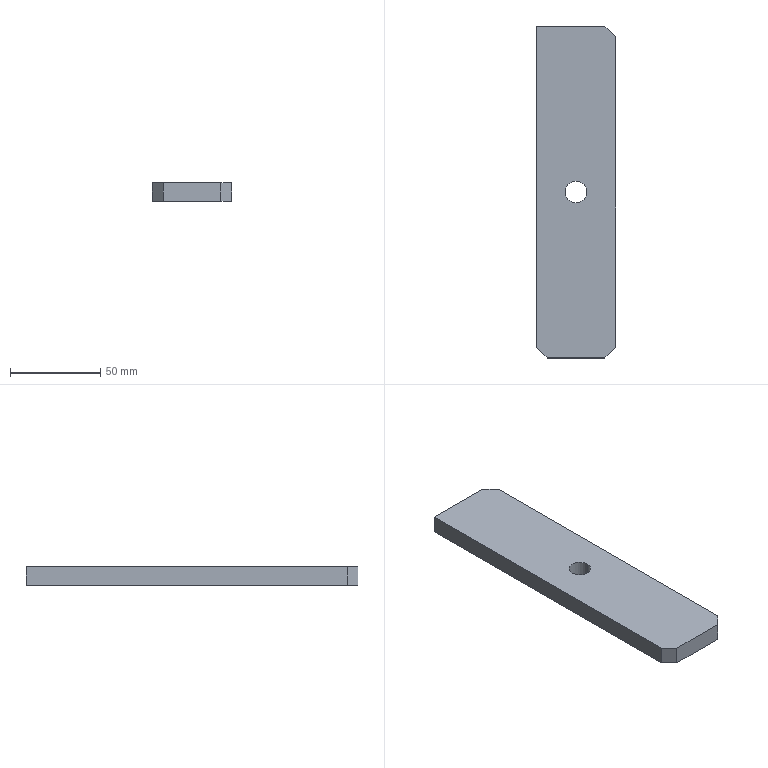Part | STEP file | PN_0011_plate_default_machined_ | 1 solid | 11 faces | box 44 x 184 x 10 mm | volume 79289 mm3 | plane 9 | cylinder 2 | commonest cylinder face diameters 12 x2
STEP:
#1=CARTESIAN_POINT('',(0.,0.,0.));
#2=DIRECTION('',(0.,0.,1.));
#3=DIRECTION('',(1.,0.,0.));
#4=AXIS2_PLACEMENT_3D('',#1,#2,#3);
#5=CARTESIAN_POINT('',(28.,92.,-10.));
#6=VERTEX_POINT('',#5);
#7=CARTESIAN_POINT('',(28.,92.,0.));
#8=VERTEX_POINT('',#7);
#9=CARTESIAN_POINT('',(28.,92.,0.));
#10=DIRECTION('',(0.,0.,1.));
#11=VECTOR('',#10,1.);
#12=LINE('',#9,#11);
#13=CARTESIAN_POINT('',(22.,92.,0.));
#14=DIRECTION('',(0.,0.,1.));
#15=DIRECTION('',(1.,0.,0.));
#16=AXIS2_PLACEMENT_3D('',#13,#14,#15);
#17=CYLINDRICAL_SURFACE('',#16,6.);
#18=CARTESIAN_POINT('',(6.283,0.));
#19=DIRECTION('',(0.,1.));
#20=VECTOR('',#19,1.);
#21=LINE('',#18,#20);
#22=(GEOMETRIC_REPRESENTATION_CONTEXT(2)PARAMETRIC_REPRESENTATION_CONTEXT()REPRESENTATION_CONTEXT('',''));
#23=DEFINITIONAL_REPRESENTATION('',(#21),#22);
#24=PCURVE('',#17,#23);
#25=CARTESIAN_POINT('',(22.,92.,0.));
#26=DIRECTION('',(0.,0.,1.));
#27=DIRECTION('',(1.,0.,0.));
#28=AXIS2_PLACEMENT_3D('',#25,#26,#27);
#29=CYLINDRICAL_SURFACE('',#28,6.);
#30=CARTESIAN_POINT('',(0.,0.));
#31=DIRECTION('',(0.,1.));
#32=VECTOR('',#31,1.);
#33=LINE('',#30,#32);
#34=(GEOMETRIC_REPRESENTATION_CONTEXT(2)PARAMETRIC_REPRESENTATION_CONTEXT()REPRESENTATION_CONTEXT('',''));
#35=DEFINITIONAL_REPRESENTATION('',(#33),#34);
#36=PCURVE('',#29,#35);
#37=SURFACE_CURVE('',#12,(#24,#36),.PCURVE_S1.);
#38=EDGE_CURVE('',#6,#8,#37,.T.);
#39=ORIENTED_EDGE('',*,*,#38,.T.);
#40=CARTESIAN_POINT('',(16.,92.,0.));
#41=VERTEX_POINT('',#40);
#42=CARTESIAN_POINT('',(22.,92.,0.));
#43=DIRECTION('',(0.,0.,1.));
#44=DIRECTION('',(1.,0.,0.));
#45=AXIS2_PLACEMENT_3D('',#42,#43,#44);
#46=CIRCLE('',#45,6.);
#47=CARTESIAN_POINT('',(0.,0.));
#48=DIRECTION('',(1.,0.));
#49=VECTOR('',#48,1.);
#50=LINE('',#47,#49);
#51=(GEOMETRIC_REPRESENTATION_CONTEXT(2)PARAMETRIC_REPRESENTATION_CONTEXT()REPRESENTATION_CONTEXT('',''));
#52=DEFINITIONAL_REPRESENTATION('',(#50),#51);
#53=PCURVE('',#17,#52);
#54=CARTESIAN_POINT('',(0.,0.,0.));
#55=DIRECTION('',(0.,0.,-1.));
#56=DIRECTION('',(-1.,0.,0.));
#57=AXIS2_PLACEMENT_3D('',#54,#55,#56);
#58=PLANE('',#57);
#59=CARTESIAN_POINT('',(-28.,92.));
#60=CARTESIAN_POINT('',(-28.,102.392));
#61=CARTESIAN_POINT('',(-19.,97.196));
#62=CARTESIAN_POINT('',(-10.,92.));
#63=CARTESIAN_POINT('',(-19.,86.804));
#64=CARTESIAN_POINT('',(-28.,81.608));
#65=CARTESIAN_POINT('',(-28.,92.));
#66=(BOUNDED_CURVE()B_SPLINE_CURVE(2,(#59,#60,#61,#62,#63,#64,#65),.UNSPECIFIED.,.T.,.F.)B_SPLINE_CURVE_WITH_KNOTS((1,2,2,2,2,1),(-2.094,0.,2.094,4.189,6.283,8.378),.UNSPECIFIED.)CURVE()GEOMETRIC_REPRESENTATION_ITEM()RATIONAL_B_SPLINE_CURVE((1.,0.5,1.,0.5,1.,0.5,1.))REPRESENTATION_ITEM(''));
#67=(GEOMETRIC_REPRESENTATION_CONTEXT(2)PARAMETRIC_REPRESENTATION_CONTEXT()REPRESENTATION_CONTEXT('',''));
#68=DEFINITIONAL_REPRESENTATION('',(#66),#67);
#69=PCURVE('',#58,#68);
#70=SURFACE_CURVE('',#46,(#53,#69),.PCURVE_S1.);
#71=EDGE_CURVE('',#41,#8,#70,.T.);
#72=ORIENTED_EDGE('',*,*,#71,.F.);
#73=CARTESIAN_POINT('',(16.,92.,-10.));
#74=VERTEX_POINT('',#73);
#75=CARTESIAN_POINT('',(16.,92.,0.));
#76=DIRECTION('',(0.,0.,1.));
#77=VECTOR('',#76,1.);
#78=LINE('',#75,#77);
#79=CARTESIAN_POINT('',(3.142,0.));
#80=DIRECTION('',(0.,1.));
#81=VECTOR('',#80,1.);
#82=LINE('',#79,#81);
#83=(GEOMETRIC_REPRESENTATION_CONTEXT(2)PARAMETRIC_REPRESENTATION_CONTEXT()REPRESENTATION_CONTEXT('',''));
#84=DEFINITIONAL_REPRESENTATION('',(#82),#83);
#85=PCURVE('',#17,#84);
#86=CARTESIAN_POINT('',(3.142,0.));
#87=DIRECTION('',(0.,1.));
#88=VECTOR('',#87,1.);
#89=LINE('',#86,#88);
#90=(GEOMETRIC_REPRESENTATION_CONTEXT(2)PARAMETRIC_REPRESENTATION_CONTEXT()REPRESENTATION_CONTEXT('',''));
#91=DEFINITIONAL_REPRESENTATION('',(#89),#90);
#92=PCURVE('',#29,#91);
#93=SURFACE_CURVE('',#78,(#85,#92),.PCURVE_S1.);
#94=EDGE_CURVE('',#74,#41,#93,.T.);
#95=ORIENTED_EDGE('',*,*,#94,.F.);
#96=CARTESIAN_POINT('',(22.,92.,-10.));
#97=DIRECTION('',(0.,0.,1.));
#98=DIRECTION('',(1.,0.,0.));
#99=AXIS2_PLACEMENT_3D('',#96,#97,#98);
#100=CIRCLE('',#99,6.);
#101=CARTESIAN_POINT('',(0.,-10.));
#102=DIRECTION('',(1.,0.));
#103=VECTOR('',#102,1.);
#104=LINE('',#101,#103);
#105=(GEOMETRIC_REPRESENTATION_CONTEXT(2)PARAMETRIC_REPRESENTATION_CONTEXT()REPRESENTATION_CONTEXT('',''));
#106=DEFINITIONAL_REPRESENTATION('',(#104),#105);
#107=PCURVE('',#17,#106);
#108=CARTESIAN_POINT('',(0.,0.,-10.));
#109=DIRECTION('',(0.,0.,-1.));
#110=DIRECTION('',(-1.,0.,0.));
#111=AXIS2_PLACEMENT_3D('',#108,#109,#110);
#112=PLANE('',#111);
#113=CARTESIAN_POINT('',(-28.,92.));
#114=CARTESIAN_POINT('',(-28.,102.392));
#115=CARTESIAN_POINT('',(-19.,97.196));
#116=CARTESIAN_POINT('',(-10.,92.));
#117=CARTESIAN_POINT('',(-19.,86.804));
#118=CARTESIAN_POINT('',(-28.,81.608));
#119=CARTESIAN_POINT('',(-28.,92.));
#120=(BOUNDED_CURVE()B_SPLINE_CURVE(2,(#113,#114,#115,#116,#117,#118,#119),.UNSPECIFIED.,.T.,.F.)B_SPLINE_CURVE_WITH_KNOTS((1,2,2,2,2,1),(-2.094,0.,2.094,4.189,6.283,8.378),.UNSPECIFIED.)CURVE()GEOMETRIC_REPRESENTATION_ITEM()RATIONAL_B_SPLINE_CURVE((1.,0.5,1.,0.5,1.,0.5,1.))REPRESENTATION_ITEM(''));
#121=(GEOMETRIC_REPRESENTATION_CONTEXT(2)PARAMETRIC_REPRESENTATION_CONTEXT()REPRESENTATION_CONTEXT('',''));
#122=DEFINITIONAL_REPRESENTATION('',(#120),#121);
#123=PCURVE('',#112,#122);
#124=SURFACE_CURVE('',#100,(#107,#123),.PCURVE_S1.);
#125=EDGE_CURVE('',#74,#6,#124,.T.);
#126=ORIENTED_EDGE('',*,*,#125,.T.);
#127=EDGE_LOOP('',(#39,#72,#95,#126));
#128=FACE_BOUND('',#127,.F.);
#129=ADVANCED_FACE('',(#128),#17,.F.);
#130=CARTESIAN_POINT('',(6.,0.,0.));
#131=VERTEX_POINT('',#130);
#132=CARTESIAN_POINT('',(0.,6.,0.));
#133=VERTEX_POINT('',#132);
#134=CARTESIAN_POINT('',(6.,0.,0.));
#135=DIRECTION('',(-0.7071,0.7071,0.));
#136=VECTOR('',#135,1.);
#137=LINE('',#134,#136);
#138=CARTESIAN_POINT('',(-6.,0.));
#139=DIRECTION('',(0.7071,0.7071));
#140=VECTOR('',#139,1.);
#141=LINE('',#138,#140);
#142=(GEOMETRIC_REPRESENTATION_CONTEXT(2)PARAMETRIC_REPRESENTATION_CONTEXT()REPRESENTATION_CONTEXT('',''));
#143=DEFINITIONAL_REPRESENTATION('',(#141),#142);
#144=PCURVE('',#58,#143);
#145=CARTESIAN_POINT('',(0.,6.,-10.));
#146=DIRECTION('',(0.7071,0.7071,0.));
#147=DIRECTION('',(-0.7071,0.7071,0.));
#148=AXIS2_PLACEMENT_3D('',#145,#146,#147);
#149=PLANE('',#148);
#150=CARTESIAN_POINT('',(-8.485,10.));
#151=DIRECTION('',(1.,0.));
#152=VECTOR('',#151,1.);
#153=LINE('',#150,#152);
#154=(GEOMETRIC_REPRESENTATION_CONTEXT(2)PARAMETRIC_REPRESENTATION_CONTEXT()REPRESENTATION_CONTEXT('',''));
#155=DEFINITIONAL_REPRESENTATION('',(#153),#154);
#156=PCURVE('',#149,#155);
#157=SURFACE_CURVE('',#137,(#144,#156),.PCURVE_S1.);
#158=EDGE_CURVE('',#131,#133,#157,.T.);
#159=ORIENTED_EDGE('',*,*,#158,.F.);
#160=CARTESIAN_POINT('',(38.,0.,0.));
#161=VERTEX_POINT('',#160);
#162=CARTESIAN_POINT('',(0.,0.,0.));
#163=DIRECTION('',(-1.,0.,0.));
#164=VECTOR('',#163,1.);
#165=LINE('',#162,#164);
#166=CARTESIAN_POINT('',(0.,0.));
#167=DIRECTION('',(1.,0.));
#168=VECTOR('',#167,1.);
#169=LINE('',#166,#168);
#170=(GEOMETRIC_REPRESENTATION_CONTEXT(2)PARAMETRIC_REPRESENTATION_CONTEXT()REPRESENTATION_CONTEXT('',''));
#171=DEFINITIONAL_REPRESENTATION('',(#169),#170);
#172=PCURVE('',#58,#171);
#173=CARTESIAN_POINT('',(0.,0.,-10.));
#174=DIRECTION('',(0.,-1.,0.));
#175=DIRECTION('',(0.,0.,-1.));
#176=AXIS2_PLACEMENT_3D('',#173,#174,#175);
#177=PLANE('',#176);
#178=CARTESIAN_POINT('',(-10.,0.));
#179=DIRECTION('',(0.,-1.));
#180=VECTOR('',#179,1.);
#181=LINE('',#178,#180);
#182=(GEOMETRIC_REPRESENTATION_CONTEXT(2)PARAMETRIC_REPRESENTATION_CONTEXT()REPRESENTATION_CONTEXT('',''));
#183=DEFINITIONAL_REPRESENTATION('',(#181),#182);
#184=PCURVE('',#177,#183);
#185=SURFACE_CURVE('',#165,(#172,#184),.PCURVE_S1.);
#186=EDGE_CURVE('',#161,#131,#185,.T.);
#187=ORIENTED_EDGE('',*,*,#186,.F.);
#188=CARTESIAN_POINT('',(44.,6.,0.));
#189=VERTEX_POINT('',#188);
#190=CARTESIAN_POINT('',(44.,6.,0.));
#191=DIRECTION('',(-0.7071,-0.7071,0.));
#192=VECTOR('',#191,1.);
#193=LINE('',#190,#192);
#194=CARTESIAN_POINT('',(-44.,6.));
#195=DIRECTION('',(0.7071,-0.7071));
#196=VECTOR('',#195,1.);
#197=LINE('',#194,#196);
#198=(GEOMETRIC_REPRESENTATION_CONTEXT(2)PARAMETRIC_REPRESENTATION_CONTEXT()REPRESENTATION_CONTEXT('',''));
#199=DEFINITIONAL_REPRESENTATION('',(#197),#198);
#200=PCURVE('',#58,#199);
#201=CARTESIAN_POINT('',(38.,0.,-10.));
#202=DIRECTION('',(-0.7071,0.7071,0.));
#203=DIRECTION('',(-0.7071,-0.7071,0.));
#204=AXIS2_PLACEMENT_3D('',#201,#202,#203);
#205=PLANE('',#204);
#206=CARTESIAN_POINT('',(-8.485,10.));
#207=DIRECTION('',(1.,0.));
#208=VECTOR('',#207,1.);
#209=LINE('',#206,#208);
#210=(GEOMETRIC_REPRESENTATION_CONTEXT(2)PARAMETRIC_REPRESENTATION_CONTEXT()REPRESENTATION_CONTEXT('',''));
#211=DEFINITIONAL_REPRESENTATION('',(#209),#210);
#212=PCURVE('',#205,#211);
#213=SURFACE_CURVE('',#193,(#200,#212),.PCURVE_S1.);
#214=EDGE_CURVE('',#189,#161,#213,.T.);
#215=ORIENTED_EDGE('',*,*,#214,.F.);
#216=CARTESIAN_POINT('',(44.,178.,0.));
#217=VERTEX_POINT('',#216);
#218=CARTESIAN_POINT('',(44.,0.,0.));
#219=DIRECTION('',(0.,-1.,0.));
#220=VECTOR('',#219,1.);
#221=LINE('',#218,#220);
#222=CARTESIAN_POINT('',(-44.,0.));
#223=DIRECTION('',(0.,-1.));
#224=VECTOR('',#223,1.);
#225=LINE('',#222,#224);
#226=(GEOMETRIC_REPRESENTATION_CONTEXT(2)PARAMETRIC_REPRESENTATION_CONTEXT()REPRESENTATION_CONTEXT('',''));
#227=DEFINITIONAL_REPRESENTATION('',(#225),#226);
#228=PCURVE('',#58,#227);
#229=CARTESIAN_POINT('',(44.,0.,-10.));
#230=DIRECTION('',(1.,0.,0.));
#231=DIRECTION('',(0.,0.,-1.));
#232=AXIS2_PLACEMENT_3D('',#229,#230,#231);
#233=PLANE('',#232);
#234=CARTESIAN_POINT('',(-10.,0.));
#235=DIRECTION('',(0.,-1.));
#236=VECTOR('',#235,1.);
#237=LINE('',#234,#236);
#238=(GEOMETRIC_REPRESENTATION_CONTEXT(2)PARAMETRIC_REPRESENTATION_CONTEXT()REPRESENTATION_CONTEXT('',''));
#239=DEFINITIONAL_REPRESENTATION('',(#237),#238);
#240=PCURVE('',#233,#239);
#241=SURFACE_CURVE('',#221,(#228,#240),.PCURVE_S1.);
#242=EDGE_CURVE('',#217,#189,#241,.T.);
#243=ORIENTED_EDGE('',*,*,#242,.F.);
#244=CARTESIAN_POINT('',(38.,184.,0.));
#245=VERTEX_POINT('',#244);
#246=CARTESIAN_POINT('',(38.,184.,0.));
#247=DIRECTION('',(0.7071,-0.7071,0.));
#248=VECTOR('',#247,1.);
#249=LINE('',#246,#248);
#250=CARTESIAN_POINT('',(-38.,184.));
#251=DIRECTION('',(-0.7071,-0.7071));
#252=VECTOR('',#251,1.);
#253=LINE('',#250,#252);
#254=(GEOMETRIC_REPRESENTATION_CONTEXT(2)PARAMETRIC_REPRESENTATION_CONTEXT()REPRESENTATION_CONTEXT('',''));
#255=DEFINITIONAL_REPRESENTATION('',(#253),#254);
#256=PCURVE('',#58,#255);
#257=CARTESIAN_POINT('',(44.,178.,-10.));
#258=DIRECTION('',(-0.7071,-0.7071,0.));
#259=DIRECTION('',(0.7071,-0.7071,0.));
#260=AXIS2_PLACEMENT_3D('',#257,#258,#259);
#261=PLANE('',#260);
#262=CARTESIAN_POINT('',(-8.485,10.));
#263=DIRECTION('',(1.,0.));
#264=VECTOR('',#263,1.);
#265=LINE('',#262,#264);
#266=(GEOMETRIC_REPRESENTATION_CONTEXT(2)PARAMETRIC_REPRESENTATION_CONTEXT()REPRESENTATION_CONTEXT('',''));
#267=DEFINITIONAL_REPRESENTATION('',(#265),#266);
#268=PCURVE('',#261,#267);
#269=SURFACE_CURVE('',#249,(#256,#268),.PCURVE_S1.);
#270=EDGE_CURVE('',#245,#217,#269,.T.);
#271=ORIENTED_EDGE('',*,*,#270,.F.);
#272=CARTESIAN_POINT('',(0.,184.,0.));
#273=VERTEX_POINT('',#272);
#274=CARTESIAN_POINT('',(0.,184.,0.));
#275=DIRECTION('',(1.,0.,0.));
#276=VECTOR('',#275,1.);
#277=LINE('',#274,#276);
#278=CARTESIAN_POINT('',(0.,184.));
#279=DIRECTION('',(-1.,0.));
#280=VECTOR('',#279,1.);
#281=LINE('',#278,#280);
#282=(GEOMETRIC_REPRESENTATION_CONTEXT(2)PARAMETRIC_REPRESENTATION_CONTEXT()REPRESENTATION_CONTEXT('',''));
#283=DEFINITIONAL_REPRESENTATION('',(#281),#282);
#284=PCURVE('',#58,#283);
#285=CARTESIAN_POINT('',(0.,184.,-10.));
#286=DIRECTION('',(0.,1.,0.));
#287=DIRECTION('',(0.,0.,1.));
#288=AXIS2_PLACEMENT_3D('',#285,#286,#287);
#289=PLANE('',#288);
#290=CARTESIAN_POINT('',(10.,0.));
#291=DIRECTION('',(0.,1.));
#292=VECTOR('',#291,1.);
#293=LINE('',#290,#292);
#294=(GEOMETRIC_REPRESENTATION_CONTEXT(2)PARAMETRIC_REPRESENTATION_CONTEXT()REPRESENTATION_CONTEXT('',''));
#295=DEFINITIONAL_REPRESENTATION('',(#293),#294);
#296=PCURVE('',#289,#295);
#297=SURFACE_CURVE('',#277,(#284,#296),.PCURVE_S1.);
#298=EDGE_CURVE('',#273,#245,#297,.T.);
#299=ORIENTED_EDGE('',*,*,#298,.F.);
#300=CARTESIAN_POINT('',(0.,0.,0.));
#301=DIRECTION('',(0.,1.,0.));
#302=VECTOR('',#301,1.);
#303=LINE('',#300,#302);
#304=CARTESIAN_POINT('',(0.,0.));
#305=DIRECTION('',(0.,1.));
#306=VECTOR('',#305,1.);
#307=LINE('',#304,#306);
#308=(GEOMETRIC_REPRESENTATION_CONTEXT(2)PARAMETRIC_REPRESENTATION_CONTEXT()REPRESENTATION_CONTEXT('',''));
#309=DEFINITIONAL_REPRESENTATION('',(#307),#308);
#310=PCURVE('',#58,#309);
#311=CARTESIAN_POINT('',(0.,0.,-10.));
#312=DIRECTION('',(-1.,0.,0.));
#313=DIRECTION('',(0.,0.,1.));
#314=AXIS2_PLACEMENT_3D('',#311,#312,#313);
#315=PLANE('',#314);
#316=CARTESIAN_POINT('',(10.,0.));
#317=DIRECTION('',(0.,1.));
#318=VECTOR('',#317,1.);
#319=LINE('',#316,#318);
#320=(GEOMETRIC_REPRESENTATION_CONTEXT(2)PARAMETRIC_REPRESENTATION_CONTEXT()REPRESENTATION_CONTEXT('',''));
#321=DEFINITIONAL_REPRESENTATION('',(#319),#320);
#322=PCURVE('',#315,#321);
#323=SURFACE_CURVE('',#303,(#310,#322),.PCURVE_S1.);
#324=EDGE_CURVE('',#133,#273,#323,.T.);
#325=ORIENTED_EDGE('',*,*,#324,.F.);
#326=EDGE_LOOP('',(#159,#187,#215,#243,#271,#299,#325));
#327=FACE_BOUND('',#326,.T.);
#328=CARTESIAN_POINT('',(22.,92.,0.));
#329=DIRECTION('',(0.,0.,1.));
#330=DIRECTION('',(1.,0.,0.));
#331=AXIS2_PLACEMENT_3D('',#328,#329,#330);
#332=CIRCLE('',#331,6.);
#333=CARTESIAN_POINT('',(-28.,92.));
#334=CARTESIAN_POINT('',(-28.,102.392));
#335=CARTESIAN_POINT('',(-19.,97.196));
#336=CARTESIAN_POINT('',(-10.,92.));
#337=CARTESIAN_POINT('',(-19.,86.804));
#338=CARTESIAN_POINT('',(-28.,81.608));
#339=CARTESIAN_POINT('',(-28.,92.));
#340=(BOUNDED_CURVE()B_SPLINE_CURVE(2,(#333,#334,#335,#336,#337,#338,#339),.UNSPECIFIED.,.T.,.F.)B_SPLINE_CURVE_WITH_KNOTS((1,2,2,2,2,1),(-2.094,0.,2.094,4.189,6.283,8.378),.UNSPECIFIED.)CURVE()GEOMETRIC_REPRESENTATION_ITEM()RATIONAL_B_SPLINE_CURVE((1.,0.5,1.,0.5,1.,0.5,1.))REPRESENTATION_ITEM(''));
#341=(GEOMETRIC_REPRESENTATION_CONTEXT(2)PARAMETRIC_REPRESENTATION_CONTEXT()REPRESENTATION_CONTEXT('',''));
#342=DEFINITIONAL_REPRESENTATION('',(#340),#341);
#343=PCURVE('',#58,#342);
#344=CARTESIAN_POINT('',(0.,0.));
#345=DIRECTION('',(1.,0.));
#346=VECTOR('',#345,1.);
#347=LINE('',#344,#346);
#348=(GEOMETRIC_REPRESENTATION_CONTEXT(2)PARAMETRIC_REPRESENTATION_CONTEXT()REPRESENTATION_CONTEXT('',''));
#349=DEFINITIONAL_REPRESENTATION('',(#347),#348);
#350=PCURVE('',#29,#349);
#351=SURFACE_CURVE('',#332,(#343,#350),.PCURVE_S1.);
#352=EDGE_CURVE('',#8,#41,#351,.T.);
#353=ORIENTED_EDGE('',*,*,#352,.F.);
#354=ORIENTED_EDGE('',*,*,#71,.F.);
#355=EDGE_LOOP('',(#353,#354));
#356=FACE_BOUND('',#355,.T.);
#357=ADVANCED_FACE('',(#327,#356),#58,.F.);
#358=ORIENTED_EDGE('',*,*,#324,.T.);
#359=CARTESIAN_POINT('',(0.,184.,-10.));
#360=VERTEX_POINT('',#359);
#361=CARTESIAN_POINT('',(0.,184.,-10.));
#362=DIRECTION('',(0.,0.,-1.));
#363=VECTOR('',#362,1.);
#364=LINE('',#361,#363);
#365=CARTESIAN_POINT('',(0.,184.));
#366=DIRECTION('',(-1.,0.));
#367=VECTOR('',#366,1.);
#368=LINE('',#365,#367);
#369=(GEOMETRIC_REPRESENTATION_CONTEXT(2)PARAMETRIC_REPRESENTATION_CONTEXT()REPRESENTATION_CONTEXT('',''));
#370=DEFINITIONAL_REPRESENTATION('',(#368),#369);
#371=PCURVE('',#315,#370);
#372=CARTESIAN_POINT('',(0.,0.));
#373=DIRECTION('',(-1.,0.));
#374=VECTOR('',#373,1.);
#375=LINE('',#372,#374);
#376=(GEOMETRIC_REPRESENTATION_CONTEXT(2)PARAMETRIC_REPRESENTATION_CONTEXT()REPRESENTATION_CONTEXT('',''));
#377=DEFINITIONAL_REPRESENTATION('',(#375),#376);
#378=PCURVE('',#289,#377);
#379=SURFACE_CURVE('',#364,(#371,#378),.PCURVE_S1.);
#380=EDGE_CURVE('',#273,#360,#379,.T.);
#381=ORIENTED_EDGE('',*,*,#380,.T.);
#382=CARTESIAN_POINT('',(0.,6.,-10.));
#383=VERTEX_POINT('',#382);
#384=CARTESIAN_POINT('',(0.,0.,-10.));
#385=DIRECTION('',(0.,-1.,0.));
#386=VECTOR('',#385,1.);
#387=LINE('',#384,#386);
#388=CARTESIAN_POINT('',(0.,0.));
#389=DIRECTION('',(0.,-1.));
#390=VECTOR('',#389,1.);
#391=LINE('',#388,#390);
#392=(GEOMETRIC_REPRESENTATION_CONTEXT(2)PARAMETRIC_REPRESENTATION_CONTEXT()REPRESENTATION_CONTEXT('',''));
#393=DEFINITIONAL_REPRESENTATION('',(#391),#392);
#394=PCURVE('',#315,#393);
#395=CARTESIAN_POINT('',(0.,0.));
#396=DIRECTION('',(0.,-1.));
#397=VECTOR('',#396,1.);
#398=LINE('',#395,#397);
#399=(GEOMETRIC_REPRESENTATION_CONTEXT(2)PARAMETRIC_REPRESENTATION_CONTEXT()REPRESENTATION_CONTEXT('',''));
#400=DEFINITIONAL_REPRESENTATION('',(#398),#399);
#401=PCURVE('',#112,#400);
#402=SURFACE_CURVE('',#387,(#394,#401),.PCURVE_S1.);
#403=EDGE_CURVE('',#360,#383,#402,.T.);
#404=ORIENTED_EDGE('',*,*,#403,.T.);
#405=CARTESIAN_POINT('',(0.,6.,-10.));
#406=DIRECTION('',(0.,0.,1.));
#407=VECTOR('',#406,1.);
#408=LINE('',#405,#407);
#409=CARTESIAN_POINT('',(0.,6.));
#410=DIRECTION('',(1.,0.));
#411=VECTOR('',#410,1.);
#412=LINE('',#409,#411);
#413=(GEOMETRIC_REPRESENTATION_CONTEXT(2)PARAMETRIC_REPRESENTATION_CONTEXT()REPRESENTATION_CONTEXT('',''));
#414=DEFINITIONAL_REPRESENTATION('',(#412),#413);
#415=PCURVE('',#315,#414);
#416=CARTESIAN_POINT('',(0.,0.));
#417=DIRECTION('',(0.,1.));
#418=VECTOR('',#417,1.);
#419=LINE('',#416,#418);
#420=(GEOMETRIC_REPRESENTATION_CONTEXT(2)PARAMETRIC_REPRESENTATION_CONTEXT()REPRESENTATION_CONTEXT('',''));
#421=DEFINITIONAL_REPRESENTATION('',(#419),#420);
#422=PCURVE('',#149,#421);
#423=SURFACE_CURVE('',#408,(#415,#422),.PCURVE_S1.);
#424=EDGE_CURVE('',#383,#133,#423,.T.);
#425=ORIENTED_EDGE('',*,*,#424,.T.);
#426=EDGE_LOOP('',(#358,#381,#404,#425));
#427=FACE_BOUND('',#426,.T.);
#428=ADVANCED_FACE('',(#427),#315,.T.);
#429=CARTESIAN_POINT('',(6.,0.,-10.));
#430=VERTEX_POINT('',#429);
#431=CARTESIAN_POINT('',(6.,0.,-10.));
#432=DIRECTION('',(0.,0.,-1.));
#433=VECTOR('',#432,1.);
#434=LINE('',#431,#433);
#435=CARTESIAN_POINT('',(-8.485,0.));
#436=DIRECTION('',(0.,-1.));
#437=VECTOR('',#436,1.);
#438=LINE('',#435,#437);
#439=(GEOMETRIC_REPRESENTATION_CONTEXT(2)PARAMETRIC_REPRESENTATION_CONTEXT()REPRESENTATION_CONTEXT('',''));
#440=DEFINITIONAL_REPRESENTATION('',(#438),#439);
#441=PCURVE('',#149,#440);
#442=CARTESIAN_POINT('',(0.,6.));
#443=DIRECTION('',(1.,0.));
#444=VECTOR('',#443,1.);
#445=LINE('',#442,#444);
#446=(GEOMETRIC_REPRESENTATION_CONTEXT(2)PARAMETRIC_REPRESENTATION_CONTEXT()REPRESENTATION_CONTEXT('',''));
#447=DEFINITIONAL_REPRESENTATION('',(#445),#446);
#448=PCURVE('',#177,#447);
#449=SURFACE_CURVE('',#434,(#441,#448),.PCURVE_S1.);
#450=EDGE_CURVE('',#131,#430,#449,.T.);
#451=ORIENTED_EDGE('',*,*,#450,.F.);
#452=ORIENTED_EDGE('',*,*,#158,.T.);
#453=ORIENTED_EDGE('',*,*,#424,.F.);
#454=CARTESIAN_POINT('',(0.,6.,-10.));
#455=DIRECTION('',(-0.7071,0.7071,0.));
#456=VECTOR('',#455,1.);
#457=LINE('',#454,#456);
#458=CARTESIAN_POINT('',(0.,0.));
#459=DIRECTION('',(1.,0.));
#460=VECTOR('',#459,1.);
#461=LINE('',#458,#460);
#462=(GEOMETRIC_REPRESENTATION_CONTEXT(2)PARAMETRIC_REPRESENTATION_CONTEXT()REPRESENTATION_CONTEXT('',''));
#463=DEFINITIONAL_REPRESENTATION('',(#461),#462);
#464=PCURVE('',#149,#463);
#465=CARTESIAN_POINT('',(0.,6.));
#466=DIRECTION('',(0.7071,0.7071));
#467=VECTOR('',#466,1.);
#468=LINE('',#465,#467);
#469=(GEOMETRIC_REPRESENTATION_CONTEXT(2)PARAMETRIC_REPRESENTATION_CONTEXT()REPRESENTATION_CONTEXT('',''));
#470=DEFINITIONAL_REPRESENTATION('',(#468),#469);
#471=PCURVE('',#112,#470);
#472=SURFACE_CURVE('',#457,(#464,#471),.PCURVE_S1.);
#473=EDGE_CURVE('',#430,#383,#472,.T.);
#474=ORIENTED_EDGE('',*,*,#473,.F.);
#475=EDGE_LOOP('',(#451,#452,#453,#474));
#476=FACE_BOUND('',#475,.T.);
#477=ADVANCED_FACE('',(#476),#149,.F.);
#478=CARTESIAN_POINT('',(38.,0.,-10.));
#479=VERTEX_POINT('',#478);
#480=CARTESIAN_POINT('',(0.,0.,-10.));
#481=DIRECTION('',(1.,0.,0.));
#482=VECTOR('',#481,1.);
#483=LINE('',#480,#482);
#484=CARTESIAN_POINT('',(0.,0.));
#485=DIRECTION('',(0.,1.));
#486=VECTOR('',#485,1.);
#487=LINE('',#484,#486);
#488=(GEOMETRIC_REPRESENTATION_CONTEXT(2)PARAMETRIC_REPRESENTATION_CONTEXT()REPRESENTATION_CONTEXT('',''));
#489=DEFINITIONAL_REPRESENTATION('',(#487),#488);
#490=PCURVE('',#177,#489);
#491=CARTESIAN_POINT('',(0.,0.));
#492=DIRECTION('',(-1.,0.));
#493=VECTOR('',#492,1.);
#494=LINE('',#491,#493);
#495=(GEOMETRIC_REPRESENTATION_CONTEXT(2)PARAMETRIC_REPRESENTATION_CONTEXT()REPRESENTATION_CONTEXT('',''));
#496=DEFINITIONAL_REPRESENTATION('',(#494),#495);
#497=PCURVE('',#112,#496);
#498=SURFACE_CURVE('',#483,(#490,#497),.PCURVE_S1.);
#499=EDGE_CURVE('',#430,#479,#498,.T.);
#500=ORIENTED_EDGE('',*,*,#499,.T.);
#501=CARTESIAN_POINT('',(38.,0.,-10.));
#502=DIRECTION('',(0.,0.,1.));
#503=VECTOR('',#502,1.);
#504=LINE('',#501,#503);
#505=CARTESIAN_POINT('',(0.,38.));
#506=DIRECTION('',(-1.,0.));
#507=VECTOR('',#506,1.);
#508=LINE('',#505,#507);
#509=(GEOMETRIC_REPRESENTATION_CONTEXT(2)PARAMETRIC_REPRESENTATION_CONTEXT()REPRESENTATION_CONTEXT('',''));
#510=DEFINITIONAL_REPRESENTATION('',(#508),#509);
#511=PCURVE('',#177,#510);
#512=CARTESIAN_POINT('',(0.,0.));
#513=DIRECTION('',(0.,1.));
#514=VECTOR('',#513,1.);
#515=LINE('',#512,#514);
#516=(GEOMETRIC_REPRESENTATION_CONTEXT(2)PARAMETRIC_REPRESENTATION_CONTEXT()REPRESENTATION_CONTEXT('',''));
#517=DEFINITIONAL_REPRESENTATION('',(#515),#516);
#518=PCURVE('',#205,#517);
#519=SURFACE_CURVE('',#504,(#511,#518),.PCURVE_S1.);
#520=EDGE_CURVE('',#479,#161,#519,.T.);
#521=ORIENTED_EDGE('',*,*,#520,.T.);
#522=ORIENTED_EDGE('',*,*,#186,.T.);
#523=ORIENTED_EDGE('',*,*,#450,.T.);
#524=EDGE_LOOP('',(#500,#521,#522,#523));
#525=FACE_BOUND('',#524,.T.);
#526=ADVANCED_FACE('',(#525),#177,.T.);
#527=CARTESIAN_POINT('',(44.,6.,-10.));
#528=VERTEX_POINT('',#527);
#529=CARTESIAN_POINT('',(44.,6.,-10.));
#530=DIRECTION('',(0.,0.,-1.));
#531=VECTOR('',#530,1.);
#532=LINE('',#529,#531);
#533=CARTESIAN_POINT('',(-8.485,0.));
#534=DIRECTION('',(0.,-1.));
#535=VECTOR('',#534,1.);
#536=LINE('',#533,#535);
#537=(GEOMETRIC_REPRESENTATION_CONTEXT(2)PARAMETRIC_REPRESENTATION_CONTEXT()REPRESENTATION_CONTEXT('',''));
#538=DEFINITIONAL_REPRESENTATION('',(#536),#537);
#539=PCURVE('',#205,#538);
#540=CARTESIAN_POINT('',(0.,6.));
#541=DIRECTION('',(1.,0.));
#542=VECTOR('',#541,1.);
#543=LINE('',#540,#542);
#544=(GEOMETRIC_REPRESENTATION_CONTEXT(2)PARAMETRIC_REPRESENTATION_CONTEXT()REPRESENTATION_CONTEXT('',''));
#545=DEFINITIONAL_REPRESENTATION('',(#543),#544);
#546=PCURVE('',#233,#545);
#547=SURFACE_CURVE('',#532,(#539,#546),.PCURVE_S1.);
#548=EDGE_CURVE('',#189,#528,#547,.T.);
#549=ORIENTED_EDGE('',*,*,#548,.F.);
#550=ORIENTED_EDGE('',*,*,#214,.T.);
#551=ORIENTED_EDGE('',*,*,#520,.F.);
#552=CARTESIAN_POINT('',(38.,0.,-10.));
#553=DIRECTION('',(-0.7071,-0.7071,0.));
#554=VECTOR('',#553,1.);
#555=LINE('',#552,#554);
#556=CARTESIAN_POINT('',(0.,0.));
#557=DIRECTION('',(1.,0.));
#558=VECTOR('',#557,1.);
#559=LINE('',#556,#558);
#560=(GEOMETRIC_REPRESENTATION_CONTEXT(2)PARAMETRIC_REPRESENTATION_CONTEXT()REPRESENTATION_CONTEXT('',''));
#561=DEFINITIONAL_REPRESENTATION('',(#559),#560);
#562=PCURVE('',#205,#561);
#563=CARTESIAN_POINT('',(-38.,0.));
#564=DIRECTION('',(0.7071,-0.7071));
#565=VECTOR('',#564,1.);
#566=LINE('',#563,#565);
#567=(GEOMETRIC_REPRESENTATION_CONTEXT(2)PARAMETRIC_REPRESENTATION_CONTEXT()REPRESENTATION_CONTEXT('',''));
#568=DEFINITIONAL_REPRESENTATION('',(#566),#567);
#569=PCURVE('',#112,#568);
#570=SURFACE_CURVE('',#555,(#562,#569),.PCURVE_S1.);
#571=EDGE_CURVE('',#528,#479,#570,.T.);
#572=ORIENTED_EDGE('',*,*,#571,.F.);
#573=EDGE_LOOP('',(#549,#550,#551,#572));
#574=FACE_BOUND('',#573,.T.);
#575=ADVANCED_FACE('',(#574),#205,.F.);
#576=CARTESIAN_POINT('',(44.,178.,-10.));
#577=VERTEX_POINT('',#576);
#578=CARTESIAN_POINT('',(44.,0.,-10.));
#579=DIRECTION('',(0.,1.,0.));
#580=VECTOR('',#579,1.);
#581=LINE('',#578,#580);
#582=CARTESIAN_POINT('',(0.,0.));
#583=DIRECTION('',(0.,1.));
#584=VECTOR('',#583,1.);
#585=LINE('',#582,#584);
#586=(GEOMETRIC_REPRESENTATION_CONTEXT(2)PARAMETRIC_REPRESENTATION_CONTEXT()REPRESENTATION_CONTEXT('',''));
#587=DEFINITIONAL_REPRESENTATION('',(#585),#586);
#588=PCURVE('',#233,#587);
#589=CARTESIAN_POINT('',(-44.,0.));
#590=DIRECTION('',(0.,1.));
#591=VECTOR('',#590,1.);
#592=LINE('',#589,#591);
#593=(GEOMETRIC_REPRESENTATION_CONTEXT(2)PARAMETRIC_REPRESENTATION_CONTEXT()REPRESENTATION_CONTEXT('',''));
#594=DEFINITIONAL_REPRESENTATION('',(#592),#593);
#595=PCURVE('',#112,#594);
#596=SURFACE_CURVE('',#581,(#588,#595),.PCURVE_S1.);
#597=EDGE_CURVE('',#528,#577,#596,.T.);
#598=ORIENTED_EDGE('',*,*,#597,.T.);
#599=CARTESIAN_POINT('',(44.,178.,-10.));
#600=DIRECTION('',(0.,0.,1.));
#601=VECTOR('',#600,1.);
#602=LINE('',#599,#601);
#603=CARTESIAN_POINT('',(0.,178.));
#604=DIRECTION('',(-1.,0.));
#605=VECTOR('',#604,1.);
#606=LINE('',#603,#605);
#607=(GEOMETRIC_REPRESENTATION_CONTEXT(2)PARAMETRIC_REPRESENTATION_CONTEXT()REPRESENTATION_CONTEXT('',''));
#608=DEFINITIONAL_REPRESENTATION('',(#606),#607);
#609=PCURVE('',#233,#608);
#610=CARTESIAN_POINT('',(0.,0.));
#611=DIRECTION('',(0.,1.));
#612=VECTOR('',#611,1.);
#613=LINE('',#610,#612);
#614=(GEOMETRIC_REPRESENTATION_CONTEXT(2)PARAMETRIC_REPRESENTATION_CONTEXT()REPRESENTATION_CONTEXT('',''));
#615=DEFINITIONAL_REPRESENTATION('',(#613),#614);
#616=PCURVE('',#261,#615);
#617=SURFACE_CURVE('',#602,(#609,#616),.PCURVE_S1.);
#618=EDGE_CURVE('',#577,#217,#617,.T.);
#619=ORIENTED_EDGE('',*,*,#618,.T.);
#620=ORIENTED_EDGE('',*,*,#242,.T.);
#621=ORIENTED_EDGE('',*,*,#548,.T.);
#622=EDGE_LOOP('',(#598,#619,#620,#621));
#623=FACE_BOUND('',#622,.T.);
#624=ADVANCED_FACE('',(#623),#233,.T.);
#625=CARTESIAN_POINT('',(38.,184.,-10.));
#626=VERTEX_POINT('',#625);
#627=CARTESIAN_POINT('',(38.,184.,-10.));
#628=DIRECTION('',(0.,0.,-1.));
#629=VECTOR('',#628,1.);
#630=LINE('',#627,#629);
#631=CARTESIAN_POINT('',(-8.485,0.));
#632=DIRECTION('',(0.,-1.));
#633=VECTOR('',#632,1.);
#634=LINE('',#631,#633);
#635=(GEOMETRIC_REPRESENTATION_CONTEXT(2)PARAMETRIC_REPRESENTATION_CONTEXT()REPRESENTATION_CONTEXT('',''));
#636=DEFINITIONAL_REPRESENTATION('',(#634),#635);
#637=PCURVE('',#261,#636);
#638=CARTESIAN_POINT('',(0.,38.));
#639=DIRECTION('',(-1.,0.));
#640=VECTOR('',#639,1.);
#641=LINE('',#638,#640);
#642=(GEOMETRIC_REPRESENTATION_CONTEXT(2)PARAMETRIC_REPRESENTATION_CONTEXT()REPRESENTATION_CONTEXT('',''));
#643=DEFINITIONAL_REPRESENTATION('',(#641),#642);
#644=PCURVE('',#289,#643);
#645=SURFACE_CURVE('',#630,(#637,#644),.PCURVE_S1.);
#646=EDGE_CURVE('',#245,#626,#645,.T.);
#647=ORIENTED_EDGE('',*,*,#646,.F.);
#648=ORIENTED_EDGE('',*,*,#270,.T.);
#649=ORIENTED_EDGE('',*,*,#618,.F.);
#650=CARTESIAN_POINT('',(44.,178.,-10.));
#651=DIRECTION('',(0.7071,-0.7071,0.));
#652=VECTOR('',#651,1.);
#653=LINE('',#650,#652);
#654=CARTESIAN_POINT('',(0.,0.));
#655=DIRECTION('',(1.,0.));
#656=VECTOR('',#655,1.);
#657=LINE('',#654,#656);
#658=(GEOMETRIC_REPRESENTATION_CONTEXT(2)PARAMETRIC_REPRESENTATION_CONTEXT()REPRESENTATION_CONTEXT('',''));
#659=DEFINITIONAL_REPRESENTATION('',(#657),#658);
#660=PCURVE('',#261,#659);
#661=CARTESIAN_POINT('',(-44.,178.));
#662=DIRECTION('',(-0.7071,-0.7071));
#663=VECTOR('',#662,1.);
#664=LINE('',#661,#663);
#665=(GEOMETRIC_REPRESENTATION_CONTEXT(2)PARAMETRIC_REPRESENTATION_CONTEXT()REPRESENTATION_CONTEXT('',''));
#666=DEFINITIONAL_REPRESENTATION('',(#664),#665);
#667=PCURVE('',#112,#666);
#668=SURFACE_CURVE('',#653,(#660,#667),.PCURVE_S1.);
#669=EDGE_CURVE('',#626,#577,#668,.T.);
#670=ORIENTED_EDGE('',*,*,#669,.F.);
#671=EDGE_LOOP('',(#647,#648,#649,#670));
#672=FACE_BOUND('',#671,.T.);
#673=ADVANCED_FACE('',(#672),#261,.F.);
#674=CARTESIAN_POINT('',(0.,184.,-10.));
#675=DIRECTION('',(-1.,0.,0.));
#676=VECTOR('',#675,1.);
#677=LINE('',#674,#676);
#678=CARTESIAN_POINT('',(0.,0.));
#679=DIRECTION('',(0.,-1.));
#680=VECTOR('',#679,1.);
#681=LINE('',#678,#680);
#682=(GEOMETRIC_REPRESENTATION_CONTEXT(2)PARAMETRIC_REPRESENTATION_CONTEXT()REPRESENTATION_CONTEXT('',''));
#683=DEFINITIONAL_REPRESENTATION('',(#681),#682);
#684=PCURVE('',#289,#683);
#685=CARTESIAN_POINT('',(0.,184.));
#686=DIRECTION('',(1.,0.));
#687=VECTOR('',#686,1.);
#688=LINE('',#685,#687);
#689=(GEOMETRIC_REPRESENTATION_CONTEXT(2)PARAMETRIC_REPRESENTATION_CONTEXT()REPRESENTATION_CONTEXT('',''));
#690=DEFINITIONAL_REPRESENTATION('',(#688),#689);
#691=PCURVE('',#112,#690);
#692=SURFACE_CURVE('',#677,(#684,#691),.PCURVE_S1.);
#693=EDGE_CURVE('',#626,#360,#692,.T.);
#694=ORIENTED_EDGE('',*,*,#693,.T.);
#695=ORIENTED_EDGE('',*,*,#380,.F.);
#696=ORIENTED_EDGE('',*,*,#298,.T.);
#697=ORIENTED_EDGE('',*,*,#646,.T.);
#698=EDGE_LOOP('',(#694,#695,#696,#697));
#699=FACE_BOUND('',#698,.T.);
#700=ADVANCED_FACE('',(#699),#289,.T.);
#701=ORIENTED_EDGE('',*,*,#352,.F.);
#702=ORIENTED_EDGE('',*,*,#38,.F.);
#703=CARTESIAN_POINT('',(22.,92.,-10.));
#704=DIRECTION('',(0.,0.,1.));
#705=DIRECTION('',(1.,0.,0.));
#706=AXIS2_PLACEMENT_3D('',#703,#704,#705);
#707=CIRCLE('',#706,6.);
#708=CARTESIAN_POINT('',(0.,-10.));
#709=DIRECTION('',(1.,0.));
#710=VECTOR('',#709,1.);
#711=LINE('',#708,#710);
#712=(GEOMETRIC_REPRESENTATION_CONTEXT(2)PARAMETRIC_REPRESENTATION_CONTEXT()REPRESENTATION_CONTEXT('',''));
#713=DEFINITIONAL_REPRESENTATION('',(#711),#712);
#714=PCURVE('',#29,#713);
#715=CARTESIAN_POINT('',(-28.,92.));
#716=CARTESIAN_POINT('',(-28.,102.392));
#717=CARTESIAN_POINT('',(-19.,97.196));
#718=CARTESIAN_POINT('',(-10.,92.));
#719=CARTESIAN_POINT('',(-19.,86.804));
#720=CARTESIAN_POINT('',(-28.,81.608));
#721=CARTESIAN_POINT('',(-28.,92.));
#722=(BOUNDED_CURVE()B_SPLINE_CURVE(2,(#715,#716,#717,#718,#719,#720,#721),.UNSPECIFIED.,.T.,.F.)B_SPLINE_CURVE_WITH_KNOTS((1,2,2,2,2,1),(-2.094,0.,2.094,4.189,6.283,8.378),.UNSPECIFIED.)CURVE()GEOMETRIC_REPRESENTATION_ITEM()RATIONAL_B_SPLINE_CURVE((1.,0.5,1.,0.5,1.,0.5,1.))REPRESENTATION_ITEM(''));
#723=(GEOMETRIC_REPRESENTATION_CONTEXT(2)PARAMETRIC_REPRESENTATION_CONTEXT()REPRESENTATION_CONTEXT('',''));
#724=DEFINITIONAL_REPRESENTATION('',(#722),#723);
#725=PCURVE('',#112,#724);
#726=SURFACE_CURVE('',#707,(#714,#725),.PCURVE_S1.);
#727=EDGE_CURVE('',#6,#74,#726,.T.);
#728=ORIENTED_EDGE('',*,*,#727,.T.);
#729=ORIENTED_EDGE('',*,*,#94,.T.);
#730=EDGE_LOOP('',(#701,#702,#728,#729));
#731=FACE_BOUND('',#730,.F.);
#732=ADVANCED_FACE('',(#731),#29,.F.);
#733=ORIENTED_EDGE('',*,*,#597,.F.);
#734=ORIENTED_EDGE('',*,*,#571,.T.);
#735=ORIENTED_EDGE('',*,*,#499,.F.);
#736=ORIENTED_EDGE('',*,*,#473,.T.);
#737=ORIENTED_EDGE('',*,*,#403,.F.);
#738=ORIENTED_EDGE('',*,*,#693,.F.);
#739=ORIENTED_EDGE('',*,*,#669,.T.);
#740=EDGE_LOOP('',(#733,#734,#735,#736,#737,#738,#739));
#741=FACE_BOUND('',#740,.T.);
#742=ORIENTED_EDGE('',*,*,#727,.T.);
#743=ORIENTED_EDGE('',*,*,#125,.T.);
#744=EDGE_LOOP('',(#742,#743));
#745=FACE_BOUND('',#744,.T.);
#746=ADVANCED_FACE('',(#741,#745),#112,.T.);
#747=CLOSED_SHELL('',(#129,#357,#428,#477,#526,#575,#624,#673,#700,#732,#746));
#748=MANIFOLD_SOLID_BREP('',#747);
#749=(LENGTH_UNIT()NAMED_UNIT(*)SI_UNIT(.MILLI.,.METRE.));
#750=UNCERTAINTY_MEASURE_WITH_UNIT(LENGTH_MEASURE(0.0000001),#749,'','');
#751=(NAMED_UNIT(*)PLANE_ANGLE_UNIT()SI_UNIT($,.RADIAN.));
#752=(NAMED_UNIT(*)SI_UNIT($,.STERADIAN.)SOLID_ANGLE_UNIT());
#753=(GEOMETRIC_REPRESENTATION_CONTEXT(3)GLOBAL_UNCERTAINTY_ASSIGNED_CONTEXT((#750))GLOBAL_UNIT_ASSIGNED_CONTEXT((#749,#751,#752))REPRESENTATION_CONTEXT('',''));
#754=ADVANCED_BREP_SHAPE_REPRESENTATION('',(#4,#748),#753);